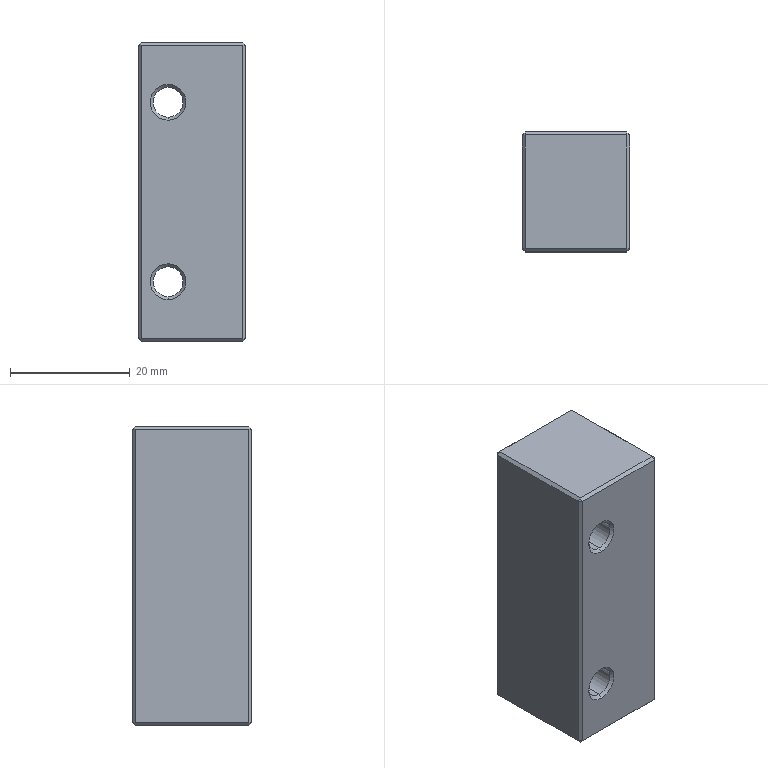Part | SolidWorks | features BaseBody 1 | 1 solid | 38 faces | box 18 x 20 x 50 mm | volume 17163 mm3 | plane 26 | cone 8 | cylinder 4 | commonest cylinder face diameters 5 x4
STEP:
#1=CARTESIAN_POINT('',(-32.,551.5,17.5));
#2=VERTEX_POINT('',#1);
#3=CARTESIAN_POINT('',(-32.,551.5,12.5));
#4=VERTEX_POINT('',#3);
#5=CARTESIAN_POINT('',(-32.,551.5,15.));
#6=DIRECTION('',(0.,-1.,0.));
#7=DIRECTION('',(0.,0.,1.));
#8=AXIS2_PLACEMENT_3D('',#5,#6,#7);
#9=CIRCLE('',#8,2.5);
#10=EDGE_CURVE('',#2,#4,#9,.T.);
#11=ORIENTED_EDGE('',*,*,#10,.F.);
#12=CARTESIAN_POINT('',(-32.,551.,18.));
#13=VERTEX_POINT('',#12);
#14=CARTESIAN_POINT('',(-32.,551.,18.));
#15=DIRECTION('',(0.,-0.7071,0.7071));
#16=VECTOR('',#15,1000.);
#17=LINE('',#14,#16);
#18=EDGE_CURVE('',#2,#13,#17,.T.);
#19=ORIENTED_EDGE('',*,*,#18,.T.);
#20=CARTESIAN_POINT('',(-32.,551.,12.));
#21=VERTEX_POINT('',#20);
#22=CARTESIAN_POINT('',(-32.,551.,15.));
#23=DIRECTION('',(0.,1.,0.));
#24=DIRECTION('',(0.,0.,1.));
#25=AXIS2_PLACEMENT_3D('',#22,#23,#24);
#26=CIRCLE('',#25,3.);
#27=EDGE_CURVE('',#21,#13,#26,.T.);
#28=ORIENTED_EDGE('',*,*,#27,.F.);
#29=CARTESIAN_POINT('',(-32.,551.,12.));
#30=DIRECTION('',(0.,-0.7071,-0.7071));
#31=VECTOR('',#30,1000.);
#32=LINE('',#29,#31);
#33=EDGE_CURVE('',#4,#21,#32,.T.);
#34=ORIENTED_EDGE('',*,*,#33,.F.);
#35=EDGE_LOOP('',(#11,#19,#28,#34));
#36=FACE_OUTER_BOUND('',#35,.T.);
#37=CARTESIAN_POINT('',(-32.,551.,15.));
#38=DIRECTION('',(0.,-1.,0.));
#39=DIRECTION('',(0.,0.,-1.));
#40=AXIS2_PLACEMENT_3D('',#37,#38,#39);
#41=CONICAL_SURFACE('',#40,3.,0.7854);
#42=ADVANCED_FACE('',(#36),#41,.F.);
#43=CARTESIAN_POINT('',(-32.,570.5,12.5));
#44=VERTEX_POINT('',#43);
#45=CARTESIAN_POINT('',(-32.,570.5,17.5));
#46=VERTEX_POINT('',#45);
#47=CARTESIAN_POINT('',(-32.,570.5,15.));
#48=DIRECTION('',(0.,1.,0.));
#49=DIRECTION('',(0.,0.,-1.));
#50=AXIS2_PLACEMENT_3D('',#47,#48,#49);
#51=CIRCLE('',#50,2.5);
#52=EDGE_CURVE('',#44,#46,#51,.T.);
#53=ORIENTED_EDGE('',*,*,#52,.F.);
#54=CARTESIAN_POINT('',(-32.,571.,12.));
#55=VERTEX_POINT('',#54);
#56=CARTESIAN_POINT('',(-32.,570.5,12.5));
#57=DIRECTION('',(0.,0.7071,-0.7071));
#58=VECTOR('',#57,1000.);
#59=LINE('',#56,#58);
#60=EDGE_CURVE('',#44,#55,#59,.T.);
#61=ORIENTED_EDGE('',*,*,#60,.T.);
#62=CARTESIAN_POINT('',(-32.,571.,18.));
#63=VERTEX_POINT('',#62);
#64=CARTESIAN_POINT('',(-32.,571.,15.));
#65=DIRECTION('',(0.,-1.,0.));
#66=DIRECTION('',(0.,0.,-1.));
#67=AXIS2_PLACEMENT_3D('',#64,#65,#66);
#68=CIRCLE('',#67,3.);
#69=EDGE_CURVE('',#63,#55,#68,.T.);
#70=ORIENTED_EDGE('',*,*,#69,.F.);
#71=CARTESIAN_POINT('',(-32.,570.5,17.5));
#72=DIRECTION('',(0.,0.7071,0.7071));
#73=VECTOR('',#72,1000.);
#74=LINE('',#71,#73);
#75=EDGE_CURVE('',#46,#63,#74,.T.);
#76=ORIENTED_EDGE('',*,*,#75,.F.);
#77=EDGE_LOOP('',(#53,#61,#70,#76));
#78=FACE_OUTER_BOUND('',#77,.T.);
#79=CARTESIAN_POINT('',(-32.,570.5,15.));
#80=DIRECTION('',(0.,1.,0.));
#81=DIRECTION('',(0.,0.,1.));
#82=AXIS2_PLACEMENT_3D('',#79,#80,#81);
#83=CONICAL_SURFACE('',#82,2.5,0.7854);
#84=ADVANCED_FACE('',(#78),#83,.F.);
#85=CARTESIAN_POINT('',(-32.,570.5,-17.5));
#86=VERTEX_POINT('',#85);
#87=CARTESIAN_POINT('',(-32.,570.5,-12.5));
#88=VERTEX_POINT('',#87);
#89=CARTESIAN_POINT('',(-32.,570.5,-15.));
#90=DIRECTION('',(0.,1.,0.));
#91=DIRECTION('',(0.,0.,-1.));
#92=AXIS2_PLACEMENT_3D('',#89,#90,#91);
#93=CIRCLE('',#92,2.5);
#94=EDGE_CURVE('',#86,#88,#93,.T.);
#95=ORIENTED_EDGE('',*,*,#94,.F.);
#96=CARTESIAN_POINT('',(-32.,571.,-18.));
#97=VERTEX_POINT('',#96);
#98=CARTESIAN_POINT('',(-32.,570.5,-17.5));
#99=DIRECTION('',(0.,0.7071,-0.7071));
#100=VECTOR('',#99,1000.);
#101=LINE('',#98,#100);
#102=EDGE_CURVE('',#86,#97,#101,.T.);
#103=ORIENTED_EDGE('',*,*,#102,.T.);
#104=CARTESIAN_POINT('',(-32.,571.,-12.));
#105=VERTEX_POINT('',#104);
#106=CARTESIAN_POINT('',(-32.,571.,-15.));
#107=DIRECTION('',(0.,-1.,0.));
#108=DIRECTION('',(0.,0.,-1.));
#109=AXIS2_PLACEMENT_3D('',#106,#107,#108);
#110=CIRCLE('',#109,3.);
#111=EDGE_CURVE('',#105,#97,#110,.T.);
#112=ORIENTED_EDGE('',*,*,#111,.F.);
#113=CARTESIAN_POINT('',(-32.,570.5,-12.5));
#114=DIRECTION('',(0.,0.7071,0.7071));
#115=VECTOR('',#114,1000.);
#116=LINE('',#113,#115);
#117=EDGE_CURVE('',#88,#105,#116,.T.);
#118=ORIENTED_EDGE('',*,*,#117,.F.);
#119=EDGE_LOOP('',(#95,#103,#112,#118));
#120=FACE_OUTER_BOUND('',#119,.T.);
#121=CARTESIAN_POINT('',(-32.,570.5,-15.));
#122=DIRECTION('',(0.,1.,0.));
#123=DIRECTION('',(0.,0.,1.));
#124=AXIS2_PLACEMENT_3D('',#121,#122,#123);
#125=CONICAL_SURFACE('',#124,2.5,0.7854);
#126=ADVANCED_FACE('',(#120),#125,.F.);
#127=CARTESIAN_POINT('',(-32.,551.5,-12.5));
#128=VERTEX_POINT('',#127);
#129=CARTESIAN_POINT('',(-32.,551.5,-17.5));
#130=VERTEX_POINT('',#129);
#131=CARTESIAN_POINT('',(-32.,551.5,-15.));
#132=DIRECTION('',(0.,-1.,0.));
#133=DIRECTION('',(0.,0.,1.));
#134=AXIS2_PLACEMENT_3D('',#131,#132,#133);
#135=CIRCLE('',#134,2.5);
#136=EDGE_CURVE('',#128,#130,#135,.T.);
#137=ORIENTED_EDGE('',*,*,#136,.F.);
#138=CARTESIAN_POINT('',(-32.,551.,-12.));
#139=VERTEX_POINT('',#138);
#140=CARTESIAN_POINT('',(-32.,551.,-12.));
#141=DIRECTION('',(0.,-0.7071,0.7071));
#142=VECTOR('',#141,1000.);
#143=LINE('',#140,#142);
#144=EDGE_CURVE('',#128,#139,#143,.T.);
#145=ORIENTED_EDGE('',*,*,#144,.T.);
#146=CARTESIAN_POINT('',(-32.,551.,-18.));
#147=VERTEX_POINT('',#146);
#148=CARTESIAN_POINT('',(-32.,551.,-15.));
#149=DIRECTION('',(0.,1.,0.));
#150=DIRECTION('',(0.,0.,1.));
#151=AXIS2_PLACEMENT_3D('',#148,#149,#150);
#152=CIRCLE('',#151,3.);
#153=EDGE_CURVE('',#147,#139,#152,.T.);
#154=ORIENTED_EDGE('',*,*,#153,.F.);
#155=CARTESIAN_POINT('',(-32.,551.,-18.));
#156=DIRECTION('',(0.,-0.7071,-0.7071));
#157=VECTOR('',#156,1000.);
#158=LINE('',#155,#157);
#159=EDGE_CURVE('',#130,#147,#158,.T.);
#160=ORIENTED_EDGE('',*,*,#159,.F.);
#161=EDGE_LOOP('',(#137,#145,#154,#160));
#162=FACE_OUTER_BOUND('',#161,.T.);
#163=CARTESIAN_POINT('',(-32.,551.,-15.));
#164=DIRECTION('',(0.,-1.,0.));
#165=DIRECTION('',(0.,0.,-1.));
#166=AXIS2_PLACEMENT_3D('',#163,#164,#165);
#167=CONICAL_SURFACE('',#166,3.,0.7854);
#168=ADVANCED_FACE('',(#162),#167,.F.);
#169=ORIENTED_EDGE('',*,*,#136,.T.);
#170=CARTESIAN_POINT('',(-32.,571.,-17.5));
#171=DIRECTION('',(0.,1.,0.));
#172=VECTOR('',#171,1000.);
#173=LINE('',#170,#172);
#174=EDGE_CURVE('',#130,#86,#173,.T.);
#175=ORIENTED_EDGE('',*,*,#174,.T.);
#176=ORIENTED_EDGE('',*,*,#94,.T.);
#177=CARTESIAN_POINT('',(-32.,571.,-12.5));
#178=DIRECTION('',(0.,1.,0.));
#179=VECTOR('',#178,1000.);
#180=LINE('',#177,#179);
#181=EDGE_CURVE('',#128,#88,#180,.T.);
#182=ORIENTED_EDGE('',*,*,#181,.F.);
#183=EDGE_LOOP('',(#169,#175,#176,#182));
#184=FACE_OUTER_BOUND('',#183,.T.);
#185=CARTESIAN_POINT('',(-32.,571.,-15.));
#186=DIRECTION('',(0.,1.,0.));
#187=DIRECTION('',(0.,0.,1.));
#188=AXIS2_PLACEMENT_3D('',#185,#186,#187);
#189=CYLINDRICAL_SURFACE('',#188,2.5);
#190=ADVANCED_FACE('',(#184),#189,.F.);
#191=ORIENTED_EDGE('',*,*,#10,.T.);
#192=CARTESIAN_POINT('',(-32.,571.,12.5));
#193=DIRECTION('',(0.,1.,0.));
#194=VECTOR('',#193,1000.);
#195=LINE('',#192,#194);
#196=EDGE_CURVE('',#4,#44,#195,.T.);
#197=ORIENTED_EDGE('',*,*,#196,.T.);
#198=ORIENTED_EDGE('',*,*,#52,.T.);
#199=CARTESIAN_POINT('',(-32.,571.,17.5));
#200=DIRECTION('',(0.,1.,0.));
#201=VECTOR('',#200,1000.);
#202=LINE('',#199,#201);
#203=EDGE_CURVE('',#2,#46,#202,.T.);
#204=ORIENTED_EDGE('',*,*,#203,.F.);
#205=EDGE_LOOP('',(#191,#197,#198,#204));
#206=FACE_OUTER_BOUND('',#205,.T.);
#207=CARTESIAN_POINT('',(-32.,571.,15.));
#208=DIRECTION('',(0.,1.,0.));
#209=DIRECTION('',(0.,0.,1.));
#210=AXIS2_PLACEMENT_3D('',#207,#208,#209);
#211=CYLINDRICAL_SURFACE('',#210,2.5);
#212=ADVANCED_FACE('',(#206),#211,.F.);
#213=CARTESIAN_POINT('',(-19.5,551.5,25.));
#214=VERTEX_POINT('',#213);
#215=CARTESIAN_POINT('',(-19.,551.5,24.5));
#216=VERTEX_POINT('',#215);
#217=CARTESIAN_POINT('',(-19.,551.5,24.5));
#218=DIRECTION('',(0.7071,0.,-0.7071));
#219=VECTOR('',#218,1000.);
#220=LINE('',#217,#219);
#221=EDGE_CURVE('',#214,#216,#220,.T.);
#222=ORIENTED_EDGE('',*,*,#221,.T.);
#223=CARTESIAN_POINT('',(-19.,570.5,24.5));
#224=VERTEX_POINT('',#223);
#225=CARTESIAN_POINT('',(-19.,551.,24.5));
#226=DIRECTION('',(0.,-1.,0.));
#227=VECTOR('',#226,1000.);
#228=LINE('',#225,#227);
#229=EDGE_CURVE('',#224,#216,#228,.T.);
#230=ORIENTED_EDGE('',*,*,#229,.F.);
#231=CARTESIAN_POINT('',(-19.5,570.5,25.));
#232=VERTEX_POINT('',#231);
#233=CARTESIAN_POINT('',(-19.5,570.5,25.));
#234=DIRECTION('',(-0.7071,0.,0.7071));
#235=VECTOR('',#234,1000.);
#236=LINE('',#233,#235);
#237=EDGE_CURVE('',#224,#232,#236,.T.);
#238=ORIENTED_EDGE('',*,*,#237,.T.);
#239=CARTESIAN_POINT('',(-19.5,571.,25.));
#240=DIRECTION('',(0.,1.,0.));
#241=VECTOR('',#240,1000.);
#242=LINE('',#239,#241);
#243=EDGE_CURVE('',#214,#232,#242,.T.);
#244=ORIENTED_EDGE('',*,*,#243,.F.);
#245=EDGE_LOOP('',(#222,#230,#238,#244));
#246=FACE_OUTER_BOUND('',#245,.T.);
#247=CARTESIAN_POINT('',(-19.5,571.,25.));
#248=DIRECTION('',(0.7071,0.,0.7071));
#249=DIRECTION('',(0.,-1.,0.));
#250=AXIS2_PLACEMENT_3D('',#247,#248,#249);
#251=PLANE('',#250);
#252=ADVANCED_FACE('',(#246),#251,.T.);
#253=CARTESIAN_POINT('',(-19.5,571.,24.5));
#254=VERTEX_POINT('',#253);
#255=CARTESIAN_POINT('',(-19.25,570.75,24.5));
#256=DIRECTION('',(-0.7071,0.7071,0.));
#257=VECTOR('',#256,1000.);
#258=LINE('',#255,#257);
#259=EDGE_CURVE('',#224,#254,#258,.T.);
#260=ORIENTED_EDGE('',*,*,#259,.T.);
#261=CARTESIAN_POINT('',(-19.5,570.5,25.));
#262=DIRECTION('',(0.,-0.7071,0.7071));
#263=VECTOR('',#262,1000.);
#264=LINE('',#261,#263);
#265=EDGE_CURVE('',#254,#232,#264,.T.);
#266=ORIENTED_EDGE('',*,*,#265,.T.);
#267=ORIENTED_EDGE('',*,*,#237,.F.);
#268=EDGE_LOOP('',(#260,#266,#267));
#269=FACE_OUTER_BOUND('',#268,.T.);
#270=CARTESIAN_POINT('',(-19.5,570.5,25.));
#271=DIRECTION('',(0.5774,0.5774,0.5774));
#272=DIRECTION('',(0.7071,0.,-0.7071));
#273=AXIS2_PLACEMENT_3D('',#270,#271,#272);
#274=PLANE('',#273);
#275=ADVANCED_FACE('',(#269),#274,.T.);
#276=CARTESIAN_POINT('',(-19.5,551.,24.5));
#277=VERTEX_POINT('',#276);
#278=CARTESIAN_POINT('',(-19.5,551.25,24.75));
#279=DIRECTION('',(0.,-0.7071,-0.7071));
#280=VECTOR('',#279,1000.);
#281=LINE('',#278,#280);
#282=EDGE_CURVE('',#214,#277,#281,.T.);
#283=ORIENTED_EDGE('',*,*,#282,.T.);
#284=CARTESIAN_POINT('',(-19.,551.5,24.5));
#285=DIRECTION('',(0.7071,0.7071,0.));
#286=VECTOR('',#285,1000.);
#287=LINE('',#284,#286);
#288=EDGE_CURVE('',#277,#216,#287,.T.);
#289=ORIENTED_EDGE('',*,*,#288,.T.);
#290=ORIENTED_EDGE('',*,*,#221,.F.);
#291=EDGE_LOOP('',(#283,#289,#290));
#292=FACE_OUTER_BOUND('',#291,.T.);
#293=CARTESIAN_POINT('',(-19.,551.5,24.5));
#294=DIRECTION('',(0.5774,-0.5774,0.5774));
#295=DIRECTION('',(0.,-0.7071,-0.7071));
#296=AXIS2_PLACEMENT_3D('',#293,#294,#295);
#297=PLANE('',#296);
#298=ADVANCED_FACE('',(#292),#297,.T.);
#299=CARTESIAN_POINT('',(-19.,570.5,-24.5));
#300=VERTEX_POINT('',#299);
#301=CARTESIAN_POINT('',(-19.5,571.,-24.5));
#302=VERTEX_POINT('',#301);
#303=CARTESIAN_POINT('',(-19.,570.5,-24.5));
#304=DIRECTION('',(-0.7071,0.7071,0.));
#305=VECTOR('',#304,1000.);
#306=LINE('',#303,#305);
#307=EDGE_CURVE('',#300,#302,#306,.T.);
#308=ORIENTED_EDGE('',*,*,#307,.T.);
#309=CARTESIAN_POINT('',(-19.5,571.,-25.));
#310=DIRECTION('',(0.,0.,-1.));
#311=VECTOR('',#310,1000.);
#312=LINE('',#309,#311);
#313=EDGE_CURVE('',#254,#302,#312,.T.);
#314=ORIENTED_EDGE('',*,*,#313,.F.);
#315=ORIENTED_EDGE('',*,*,#259,.F.);
#316=CARTESIAN_POINT('',(-19.,570.5,25.));
#317=DIRECTION('',(0.,0.,1.));
#318=VECTOR('',#317,1000.);
#319=LINE('',#316,#318);
#320=EDGE_CURVE('',#300,#224,#319,.T.);
#321=ORIENTED_EDGE('',*,*,#320,.F.);
#322=EDGE_LOOP('',(#308,#314,#315,#321));
#323=FACE_OUTER_BOUND('',#322,.T.);
#324=CARTESIAN_POINT('',(-19.5,571.,25.));
#325=DIRECTION('',(0.7071,0.7071,0.));
#326=DIRECTION('',(0.,0.,-1.));
#327=AXIS2_PLACEMENT_3D('',#324,#325,#326);
#328=PLANE('',#327);
#329=ADVANCED_FACE('',(#323),#328,.T.);
#330=CARTESIAN_POINT('',(-36.5,571.,24.5));
#331=VERTEX_POINT('',#330);
#332=CARTESIAN_POINT('',(-36.5,570.5,25.));
#333=VERTEX_POINT('',#332);
#334=CARTESIAN_POINT('',(-36.5,571.,24.5));
#335=DIRECTION('',(0.,-0.7071,0.7071));
#336=VECTOR('',#335,1000.);
#337=LINE('',#334,#336);
#338=EDGE_CURVE('',#331,#333,#337,.T.);
#339=ORIENTED_EDGE('',*,*,#338,.T.);
#340=CARTESIAN_POINT('',(-31.,570.5,25.));
#341=DIRECTION('',(-1.,0.,0.));
#342=VECTOR('',#341,1000.);
#343=LINE('',#340,#342);
#344=EDGE_CURVE('',#232,#333,#343,.T.);
#345=ORIENTED_EDGE('',*,*,#344,.F.);
#346=ORIENTED_EDGE('',*,*,#265,.F.);
#347=CARTESIAN_POINT('',(-31.,571.,24.5));
#348=DIRECTION('',(1.,0.,0.));
#349=VECTOR('',#348,1000.);
#350=LINE('',#347,#349);
#351=EDGE_CURVE('',#331,#254,#350,.T.);
#352=ORIENTED_EDGE('',*,*,#351,.F.);
#353=EDGE_LOOP('',(#339,#345,#346,#352));
#354=FACE_OUTER_BOUND('',#353,.T.);
#355=CARTESIAN_POINT('',(-31.,571.,24.5));
#356=DIRECTION('',(0.,-0.7071,-0.7071));
#357=DIRECTION('',(0.,0.7071,-0.7071));
#358=AXIS2_PLACEMENT_3D('',#355,#356,#357);
#359=PLANE('',#358);
#360=ADVANCED_FACE('',(#354),#359,.F.);
#361=CARTESIAN_POINT('',(-36.5,551.5,25.));
#362=VERTEX_POINT('',#361);
#363=CARTESIAN_POINT('',(-36.5,551.,24.5));
#364=VERTEX_POINT('',#363);
#365=CARTESIAN_POINT('',(-36.5,551.25,24.75));
#366=DIRECTION('',(0.,-0.7071,-0.7071));
#367=VECTOR('',#366,1000.);
#368=LINE('',#365,#367);
#369=EDGE_CURVE('',#362,#364,#368,.T.);
#370=ORIENTED_EDGE('',*,*,#369,.T.);
#371=CARTESIAN_POINT('',(-31.,551.,24.5));
#372=DIRECTION('',(-1.,0.,0.));
#373=VECTOR('',#372,1000.);
#374=LINE('',#371,#373);
#375=EDGE_CURVE('',#277,#364,#374,.T.);
#376=ORIENTED_EDGE('',*,*,#375,.F.);
#377=ORIENTED_EDGE('',*,*,#282,.F.);
#378=CARTESIAN_POINT('',(-31.,551.5,25.));
#379=DIRECTION('',(1.,0.,0.));
#380=VECTOR('',#379,1000.);
#381=LINE('',#378,#380);
#382=EDGE_CURVE('',#362,#214,#381,.T.);
#383=ORIENTED_EDGE('',*,*,#382,.F.);
#384=EDGE_LOOP('',(#370,#376,#377,#383));
#385=FACE_OUTER_BOUND('',#384,.T.);
#386=CARTESIAN_POINT('',(-31.,551.5,25.));
#387=DIRECTION('',(0.,0.7071,-0.7071));
#388=DIRECTION('',(-1.,0.,0.));
#389=AXIS2_PLACEMENT_3D('',#386,#387,#388);
#390=PLANE('',#389);
#391=ADVANCED_FACE('',(#385),#390,.F.);
#392=CARTESIAN_POINT('',(-19.5,551.,-24.5));
#393=VERTEX_POINT('',#392);
#394=CARTESIAN_POINT('',(-19.,551.5,-24.5));
#395=VERTEX_POINT('',#394);
#396=CARTESIAN_POINT('',(-19.,551.5,-24.5));
#397=DIRECTION('',(0.7071,0.7071,0.));
#398=VECTOR('',#397,1000.);
#399=LINE('',#396,#398);
#400=EDGE_CURVE('',#393,#395,#399,.T.);
#401=ORIENTED_EDGE('',*,*,#400,.T.);
#402=CARTESIAN_POINT('',(-19.,551.5,-25.));
#403=DIRECTION('',(0.,0.,-1.));
#404=VECTOR('',#403,1000.);
#405=LINE('',#402,#404);
#406=EDGE_CURVE('',#216,#395,#405,.T.);
#407=ORIENTED_EDGE('',*,*,#406,.F.);
#408=ORIENTED_EDGE('',*,*,#288,.F.);
#409=CARTESIAN_POINT('',(-19.5,551.,25.));
#410=DIRECTION('',(0.,0.,1.));
#411=VECTOR('',#410,1000.);
#412=LINE('',#409,#411);
#413=EDGE_CURVE('',#393,#277,#412,.T.);
#414=ORIENTED_EDGE('',*,*,#413,.F.);
#415=EDGE_LOOP('',(#401,#407,#408,#414));
#416=FACE_OUTER_BOUND('',#415,.T.);
#417=CARTESIAN_POINT('',(-19.5,551.,25.));
#418=DIRECTION('',(0.7071,-0.7071,0.));
#419=DIRECTION('',(0.,0.,-1.));
#420=AXIS2_PLACEMENT_3D('',#417,#418,#419);
#421=PLANE('',#420);
#422=ADVANCED_FACE('',(#416),#421,.T.);
#423=CARTESIAN_POINT('',(-19.5,570.5,-25.));
#424=VERTEX_POINT('',#423);
#425=CARTESIAN_POINT('',(-19.,570.5,-24.5));
#426=DIRECTION('',(-0.7071,0.,-0.7071));
#427=VECTOR('',#426,1000.);
#428=LINE('',#425,#427);
#429=EDGE_CURVE('',#300,#424,#428,.T.);
#430=ORIENTED_EDGE('',*,*,#429,.T.);
#431=CARTESIAN_POINT('',(-19.5,570.75,-24.75));
#432=DIRECTION('',(0.,0.7071,0.7071));
#433=VECTOR('',#432,1000.);
#434=LINE('',#431,#433);
#435=EDGE_CURVE('',#424,#302,#434,.T.);
#436=ORIENTED_EDGE('',*,*,#435,.T.);
#437=ORIENTED_EDGE('',*,*,#307,.F.);
#438=EDGE_LOOP('',(#430,#436,#437));
#439=FACE_OUTER_BOUND('',#438,.T.);
#440=CARTESIAN_POINT('',(-19.,570.5,-24.5));
#441=DIRECTION('',(0.5774,0.5774,-0.5774));
#442=DIRECTION('',(-0.7071,0.,-0.7071));
#443=AXIS2_PLACEMENT_3D('',#440,#441,#442);
#444=PLANE('',#443);
#445=ADVANCED_FACE('',(#439),#444,.T.);
#446=CARTESIAN_POINT('',(-37.,570.5,24.5));
#447=VERTEX_POINT('',#446);
#448=CARTESIAN_POINT('',(-36.5,571.,24.5));
#449=DIRECTION('',(-0.7071,-0.7071,0.));
#450=VECTOR('',#449,1000.);
#451=LINE('',#448,#450);
#452=EDGE_CURVE('',#331,#447,#451,.T.);
#453=ORIENTED_EDGE('',*,*,#452,.T.);
#454=CARTESIAN_POINT('',(-36.75,570.5,24.75));
#455=DIRECTION('',(0.7071,0.,0.7071));
#456=VECTOR('',#455,1000.);
#457=LINE('',#454,#456);
#458=EDGE_CURVE('',#447,#333,#457,.T.);
#459=ORIENTED_EDGE('',*,*,#458,.T.);
#460=ORIENTED_EDGE('',*,*,#338,.F.);
#461=EDGE_LOOP('',(#453,#459,#460));
#462=FACE_OUTER_BOUND('',#461,.T.);
#463=CARTESIAN_POINT('',(-36.5,571.,24.5));
#464=DIRECTION('',(-0.5774,0.5774,0.5774));
#465=DIRECTION('',(0.7071,0.,0.7071));
#466=AXIS2_PLACEMENT_3D('',#463,#464,#465);
#467=PLANE('',#466);
#468=ADVANCED_FACE('',(#462),#467,.T.);
#469=CARTESIAN_POINT('',(-37.,551.5,24.5));
#470=VERTEX_POINT('',#469);
#471=CARTESIAN_POINT('',(-37.,551.5,24.5));
#472=DIRECTION('',(-0.7071,0.,-0.7071));
#473=VECTOR('',#472,1000.);
#474=LINE('',#471,#473);
#475=EDGE_CURVE('',#362,#470,#474,.T.);
#476=ORIENTED_EDGE('',*,*,#475,.T.);
#477=CARTESIAN_POINT('',(-37.,551.5,24.5));
#478=DIRECTION('',(0.7071,-0.7071,0.));
#479=VECTOR('',#478,1000.);
#480=LINE('',#477,#479);
#481=EDGE_CURVE('',#470,#364,#480,.T.);
#482=ORIENTED_EDGE('',*,*,#481,.T.);
#483=ORIENTED_EDGE('',*,*,#369,.F.);
#484=EDGE_LOOP('',(#476,#482,#483));
#485=FACE_OUTER_BOUND('',#484,.T.);
#486=CARTESIAN_POINT('',(-37.,551.5,24.5));
#487=DIRECTION('',(-0.5774,-0.5774,0.5774));
#488=DIRECTION('',(-0.7071,0.7071,0.));
#489=AXIS2_PLACEMENT_3D('',#486,#487,#488);
#490=PLANE('',#489);
#491=ADVANCED_FACE('',(#485),#490,.T.);
#492=CARTESIAN_POINT('',(-19.5,551.5,-25.));
#493=VERTEX_POINT('',#492);
#494=CARTESIAN_POINT('',(-19.5,551.25,-24.75));
#495=DIRECTION('',(0.,0.7071,-0.7071));
#496=VECTOR('',#495,1000.);
#497=LINE('',#494,#496);
#498=EDGE_CURVE('',#393,#493,#497,.T.);
#499=ORIENTED_EDGE('',*,*,#498,.T.);
#500=CARTESIAN_POINT('',(-19.,551.5,-24.5));
#501=DIRECTION('',(0.7071,0.,0.7071));
#502=VECTOR('',#501,1000.);
#503=LINE('',#500,#502);
#504=EDGE_CURVE('',#493,#395,#503,.T.);
#505=ORIENTED_EDGE('',*,*,#504,.T.);
#506=ORIENTED_EDGE('',*,*,#400,.F.);
#507=EDGE_LOOP('',(#499,#505,#506));
#508=FACE_OUTER_BOUND('',#507,.T.);
#509=CARTESIAN_POINT('',(-19.,551.5,-24.5));
#510=DIRECTION('',(0.5774,-0.5774,-0.5774));
#511=DIRECTION('',(0.,0.7071,-0.7071));
#512=AXIS2_PLACEMENT_3D('',#509,#510,#511);
#513=PLANE('',#512);
#514=ADVANCED_FACE('',(#508),#513,.T.);
#515=ORIENTED_EDGE('',*,*,#504,.F.);
#516=CARTESIAN_POINT('',(-19.5,551.,-25.));
#517=DIRECTION('',(0.,-1.,0.));
#518=VECTOR('',#517,1000.);
#519=LINE('',#516,#518);
#520=EDGE_CURVE('',#424,#493,#519,.T.);
#521=ORIENTED_EDGE('',*,*,#520,.F.);
#522=ORIENTED_EDGE('',*,*,#429,.F.);
#523=CARTESIAN_POINT('',(-19.,571.,-24.5));
#524=DIRECTION('',(0.,1.,0.));
#525=VECTOR('',#524,1000.);
#526=LINE('',#523,#525);
#527=EDGE_CURVE('',#395,#300,#526,.T.);
#528=ORIENTED_EDGE('',*,*,#527,.F.);
#529=EDGE_LOOP('',(#515,#521,#522,#528));
#530=FACE_OUTER_BOUND('',#529,.T.);
#531=CARTESIAN_POINT('',(-19.5,571.,-25.));
#532=DIRECTION('',(0.7071,0.,-0.7071));
#533=DIRECTION('',(0.,-1.,0.));
#534=AXIS2_PLACEMENT_3D('',#531,#532,#533);
#535=PLANE('',#534);
#536=ADVANCED_FACE('',(#530),#535,.T.);
#537=CARTESIAN_POINT('',(-36.5,570.5,-25.));
#538=VERTEX_POINT('',#537);
#539=CARTESIAN_POINT('',(-36.5,571.,-24.5));
#540=VERTEX_POINT('',#539);
#541=CARTESIAN_POINT('',(-36.5,570.5,-25.));
#542=DIRECTION('',(0.,0.7071,0.7071));
#543=VECTOR('',#542,1000.);
#544=LINE('',#541,#543);
#545=EDGE_CURVE('',#538,#540,#544,.T.);
#546=ORIENTED_EDGE('',*,*,#545,.T.);
#547=CARTESIAN_POINT('',(-31.,571.,-24.5));
#548=DIRECTION('',(-1.,0.,0.));
#549=VECTOR('',#548,1000.);
#550=LINE('',#547,#549);
#551=EDGE_CURVE('',#302,#540,#550,.T.);
#552=ORIENTED_EDGE('',*,*,#551,.F.);
#553=ORIENTED_EDGE('',*,*,#435,.F.);
#554=CARTESIAN_POINT('',(-31.,570.5,-25.));
#555=DIRECTION('',(1.,0.,0.));
#556=VECTOR('',#555,1000.);
#557=LINE('',#554,#556);
#558=EDGE_CURVE('',#538,#424,#557,.T.);
#559=ORIENTED_EDGE('',*,*,#558,.F.);
#560=EDGE_LOOP('',(#546,#552,#553,#559));
#561=FACE_OUTER_BOUND('',#560,.T.);
#562=CARTESIAN_POINT('',(-31.,570.5,-25.));
#563=DIRECTION('',(0.,-0.7071,0.7071));
#564=DIRECTION('',(-1.,0.,0.));
#565=AXIS2_PLACEMENT_3D('',#562,#563,#564);
#566=PLANE('',#565);
#567=ADVANCED_FACE('',(#561),#566,.F.);
#568=CARTESIAN_POINT('',(-37.,570.5,-24.5));
#569=VERTEX_POINT('',#568);
#570=CARTESIAN_POINT('',(-36.75,570.75,-24.5));
#571=DIRECTION('',(-0.7071,-0.7071,0.));
#572=VECTOR('',#571,1000.);
#573=LINE('',#570,#572);
#574=EDGE_CURVE('',#540,#569,#573,.T.);
#575=ORIENTED_EDGE('',*,*,#574,.T.);
#576=CARTESIAN_POINT('',(-37.,570.5,-25.));
#577=DIRECTION('',(0.,0.,-1.));
#578=VECTOR('',#577,1000.);
#579=LINE('',#576,#578);
#580=EDGE_CURVE('',#447,#569,#579,.T.);
#581=ORIENTED_EDGE('',*,*,#580,.F.);
#582=ORIENTED_EDGE('',*,*,#452,.F.);
#583=CARTESIAN_POINT('',(-36.5,571.,25.));
#584=DIRECTION('',(0.,0.,1.));
#585=VECTOR('',#584,1000.);
#586=LINE('',#583,#585);
#587=EDGE_CURVE('',#540,#331,#586,.T.);
#588=ORIENTED_EDGE('',*,*,#587,.F.);
#589=EDGE_LOOP('',(#575,#581,#582,#588));
#590=FACE_OUTER_BOUND('',#589,.T.);
#591=CARTESIAN_POINT('',(-37.,570.5,0.));
#592=DIRECTION('',(-0.7071,0.7071,0.));
#593=DIRECTION('',(0.,0.,1.));
#594=AXIS2_PLACEMENT_3D('',#591,#592,#593);
#595=PLANE('',#594);
#596=ADVANCED_FACE('',(#590),#595,.T.);
#597=ORIENTED_EDGE('',*,*,#458,.F.);
#598=CARTESIAN_POINT('',(-37.,571.,24.5));
#599=DIRECTION('',(0.,1.,0.));
#600=VECTOR('',#599,1000.);
#601=LINE('',#598,#600);
#602=EDGE_CURVE('',#470,#447,#601,.T.);
#603=ORIENTED_EDGE('',*,*,#602,.F.);
#604=ORIENTED_EDGE('',*,*,#475,.F.);
#605=CARTESIAN_POINT('',(-36.5,551.,25.));
#606=DIRECTION('',(0.,-1.,0.));
#607=VECTOR('',#606,1000.);
#608=LINE('',#605,#607);
#609=EDGE_CURVE('',#333,#362,#608,.T.);
#610=ORIENTED_EDGE('',*,*,#609,.F.);
#611=EDGE_LOOP('',(#597,#603,#604,#610));
#612=FACE_OUTER_BOUND('',#611,.T.);
#613=CARTESIAN_POINT('',(-37.,725.,24.5));
#614=DIRECTION('',(-0.7071,0.,0.7071));
#615=DIRECTION('',(0.,1.,0.));
#616=AXIS2_PLACEMENT_3D('',#613,#614,#615);
#617=PLANE('',#616);
#618=ADVANCED_FACE('',(#612),#617,.T.);
#619=CARTESIAN_POINT('',(-37.,551.5,-24.5));
#620=VERTEX_POINT('',#619);
#621=CARTESIAN_POINT('',(-36.5,551.,-24.5));
#622=VERTEX_POINT('',#621);
#623=CARTESIAN_POINT('',(-36.5,551.,-24.5));
#624=DIRECTION('',(0.7071,-0.7071,0.));
#625=VECTOR('',#624,1000.);
#626=LINE('',#623,#625);
#627=EDGE_CURVE('',#620,#622,#626,.T.);
#628=ORIENTED_EDGE('',*,*,#627,.T.);
#629=CARTESIAN_POINT('',(-36.5,551.,-25.));
#630=DIRECTION('',(0.,0.,-1.));
#631=VECTOR('',#630,1000.);
#632=LINE('',#629,#631);
#633=EDGE_CURVE('',#364,#622,#632,.T.);
#634=ORIENTED_EDGE('',*,*,#633,.F.);
#635=ORIENTED_EDGE('',*,*,#481,.F.);
#636=CARTESIAN_POINT('',(-37.,551.5,25.));
#637=DIRECTION('',(0.,0.,1.));
#638=VECTOR('',#637,1000.);
#639=LINE('',#636,#638);
#640=EDGE_CURVE('',#620,#470,#639,.T.);
#641=ORIENTED_EDGE('',*,*,#640,.F.);
#642=EDGE_LOOP('',(#628,#634,#635,#641));
#643=FACE_OUTER_BOUND('',#642,.T.);
#644=CARTESIAN_POINT('',(-37.,551.5,0.));
#645=DIRECTION('',(-0.7071,-0.7071,0.));
#646=DIRECTION('',(-0.7071,0.7071,0.));
#647=AXIS2_PLACEMENT_3D('',#644,#645,#646);
#648=PLANE('',#647);
#649=ADVANCED_FACE('',(#643),#648,.T.);
#650=CARTESIAN_POINT('',(-36.5,551.5,-25.));
#651=VERTEX_POINT('',#650);
#652=CARTESIAN_POINT('',(-36.5,551.,-24.5));
#653=DIRECTION('',(0.,0.7071,-0.7071));
#654=VECTOR('',#653,1000.);
#655=LINE('',#652,#654);
#656=EDGE_CURVE('',#622,#651,#655,.T.);
#657=ORIENTED_EDGE('',*,*,#656,.T.);
#658=CARTESIAN_POINT('',(-31.,551.5,-25.));
#659=DIRECTION('',(-1.,0.,0.));
#660=VECTOR('',#659,1000.);
#661=LINE('',#658,#660);
#662=EDGE_CURVE('',#493,#651,#661,.T.);
#663=ORIENTED_EDGE('',*,*,#662,.F.);
#664=ORIENTED_EDGE('',*,*,#498,.F.);
#665=CARTESIAN_POINT('',(-31.,551.,-24.5));
#666=DIRECTION('',(1.,0.,0.));
#667=VECTOR('',#666,1000.);
#668=LINE('',#665,#667);
#669=EDGE_CURVE('',#622,#393,#668,.T.);
#670=ORIENTED_EDGE('',*,*,#669,.F.);
#671=EDGE_LOOP('',(#657,#663,#664,#670));
#672=FACE_OUTER_BOUND('',#671,.T.);
#673=CARTESIAN_POINT('',(-31.,551.,-24.5));
#674=DIRECTION('',(0.,0.7071,0.7071));
#675=DIRECTION('',(1.,0.,0.));
#676=AXIS2_PLACEMENT_3D('',#673,#674,#675);
#677=PLANE('',#676);
#678=ADVANCED_FACE('',(#672),#677,.F.);
#679=ORIENTED_EDGE('',*,*,#545,.F.);
#680=CARTESIAN_POINT('',(-36.5,570.5,-25.));
#681=DIRECTION('',(-0.7071,0.,0.7071));
#682=VECTOR('',#681,1000.);
#683=LINE('',#680,#682);
#684=EDGE_CURVE('',#538,#569,#683,.T.);
#685=ORIENTED_EDGE('',*,*,#684,.T.);
#686=ORIENTED_EDGE('',*,*,#574,.F.);
#687=EDGE_LOOP('',(#679,#685,#686));
#688=FACE_OUTER_BOUND('',#687,.T.);
#689=CARTESIAN_POINT('',(-36.5,570.5,-25.));
#690=DIRECTION('',(-0.5774,0.5774,-0.5774));
#691=DIRECTION('',(-0.7071,0.,0.7071));
#692=AXIS2_PLACEMENT_3D('',#689,#690,#691);
#693=PLANE('',#692);
#694=ADVANCED_FACE('',(#688),#693,.T.);
#695=ORIENTED_EDGE('',*,*,#627,.F.);
#696=CARTESIAN_POINT('',(-36.75,551.5,-24.75));
#697=DIRECTION('',(0.7071,0.,-0.7071));
#698=VECTOR('',#697,1000.);
#699=LINE('',#696,#698);
#700=EDGE_CURVE('',#620,#651,#699,.T.);
#701=ORIENTED_EDGE('',*,*,#700,.T.);
#702=ORIENTED_EDGE('',*,*,#656,.F.);
#703=EDGE_LOOP('',(#695,#701,#702));
#704=FACE_OUTER_BOUND('',#703,.T.);
#705=CARTESIAN_POINT('',(-36.5,551.,-24.5));
#706=DIRECTION('',(-0.5774,-0.5774,-0.5774));
#707=DIRECTION('',(-0.7071,0.7071,0.));
#708=AXIS2_PLACEMENT_3D('',#705,#706,#707);
#709=PLANE('',#708);
#710=ADVANCED_FACE('',(#704),#709,.T.);
#711=ORIENTED_EDGE('',*,*,#700,.F.);
#712=CARTESIAN_POINT('',(-37.,551.,-24.5));
#713=DIRECTION('',(0.,-1.,0.));
#714=VECTOR('',#713,1000.);
#715=LINE('',#712,#714);
#716=EDGE_CURVE('',#569,#620,#715,.T.);
#717=ORIENTED_EDGE('',*,*,#716,.F.);
#718=ORIENTED_EDGE('',*,*,#684,.F.);
#719=CARTESIAN_POINT('',(-36.5,571.,-25.));
#720=DIRECTION('',(0.,1.,0.));
#721=VECTOR('',#720,1000.);
#722=LINE('',#719,#721);
#723=EDGE_CURVE('',#651,#538,#722,.T.);
#724=ORIENTED_EDGE('',*,*,#723,.F.);
#725=EDGE_LOOP('',(#711,#717,#718,#724));
#726=FACE_OUTER_BOUND('',#725,.T.);
#727=CARTESIAN_POINT('',(-37.,725.,-24.5));
#728=DIRECTION('',(-0.7071,0.,-0.7071));
#729=DIRECTION('',(-0.7071,0.,0.7071));
#730=AXIS2_PLACEMENT_3D('',#727,#728,#729);
#731=PLANE('',#730);
#732=ADVANCED_FACE('',(#726),#731,.T.);
#733=ORIENTED_EDGE('',*,*,#320,.T.);
#734=ORIENTED_EDGE('',*,*,#229,.T.);
#735=ORIENTED_EDGE('',*,*,#406,.T.);
#736=ORIENTED_EDGE('',*,*,#527,.T.);
#737=EDGE_LOOP('',(#733,#734,#735,#736));
#738=FACE_OUTER_BOUND('',#737,.T.);
#739=CARTESIAN_POINT('',(-19.,0.,0.));
#740=DIRECTION('',(1.,0.,0.));
#741=DIRECTION('',(0.,1.,0.));
#742=AXIS2_PLACEMENT_3D('',#739,#740,#741);
#743=PLANE('',#742);
#744=ADVANCED_FACE('',(#738),#743,.T.);
#745=ORIENTED_EDGE('',*,*,#716,.T.);
#746=ORIENTED_EDGE('',*,*,#640,.T.);
#747=ORIENTED_EDGE('',*,*,#602,.T.);
#748=ORIENTED_EDGE('',*,*,#580,.T.);
#749=EDGE_LOOP('',(#745,#746,#747,#748));
#750=FACE_OUTER_BOUND('',#749,.T.);
#751=CARTESIAN_POINT('',(-37.,725.,0.));
#752=DIRECTION('',(-1.,0.,0.));
#753=DIRECTION('',(0.,0.,1.));
#754=AXIS2_PLACEMENT_3D('',#751,#752,#753);
#755=PLANE('',#754);
#756=ADVANCED_FACE('',(#750),#755,.T.);
#757=ORIENTED_EDGE('',*,*,#27,.T.);
#758=CARTESIAN_POINT('',(-32.,551.,15.));
#759=DIRECTION('',(0.,1.,0.));
#760=DIRECTION('',(0.,0.,1.));
#761=AXIS2_PLACEMENT_3D('',#758,#759,#760);
#762=CIRCLE('',#761,3.);
#763=EDGE_CURVE('',#13,#21,#762,.T.);
#764=ORIENTED_EDGE('',*,*,#763,.T.);
#765=EDGE_LOOP('',(#757,#764));
#766=FACE_BOUND('',#765,.T.);
#767=ORIENTED_EDGE('',*,*,#153,.T.);
#768=CARTESIAN_POINT('',(-32.,551.,-15.));
#769=DIRECTION('',(0.,1.,0.));
#770=DIRECTION('',(0.,0.,1.));
#771=AXIS2_PLACEMENT_3D('',#768,#769,#770);
#772=CIRCLE('',#771,3.);
#773=EDGE_CURVE('',#139,#147,#772,.T.);
#774=ORIENTED_EDGE('',*,*,#773,.T.);
#775=EDGE_LOOP('',(#767,#774));
#776=FACE_BOUND('',#775,.T.);
#777=ORIENTED_EDGE('',*,*,#633,.T.);
#778=ORIENTED_EDGE('',*,*,#669,.T.);
#779=ORIENTED_EDGE('',*,*,#413,.T.);
#780=ORIENTED_EDGE('',*,*,#375,.T.);
#781=EDGE_LOOP('',(#777,#778,#779,#780));
#782=FACE_OUTER_BOUND('',#781,.T.);
#783=CARTESIAN_POINT('',(-31.,551.,25.));
#784=DIRECTION('',(0.,1.,0.));
#785=DIRECTION('',(1.,0.,0.));
#786=AXIS2_PLACEMENT_3D('',#783,#784,#785);
#787=PLANE('',#786);
#788=ADVANCED_FACE('',(#766,#776,#782),#787,.F.);
#789=ORIENTED_EDGE('',*,*,#558,.T.);
#790=ORIENTED_EDGE('',*,*,#520,.T.);
#791=ORIENTED_EDGE('',*,*,#662,.T.);
#792=ORIENTED_EDGE('',*,*,#723,.T.);
#793=EDGE_LOOP('',(#789,#790,#791,#792));
#794=FACE_OUTER_BOUND('',#793,.T.);
#795=CARTESIAN_POINT('',(-31.,571.,-25.));
#796=DIRECTION('',(0.,0.,1.));
#797=DIRECTION('',(1.,0.,0.));
#798=AXIS2_PLACEMENT_3D('',#795,#796,#797);
#799=PLANE('',#798);
#800=ADVANCED_FACE('',(#794),#799,.F.);
#801=ORIENTED_EDGE('',*,*,#69,.T.);
#802=CARTESIAN_POINT('',(-32.,571.,15.));
#803=DIRECTION('',(0.,-1.,0.));
#804=DIRECTION('',(0.,0.,-1.));
#805=AXIS2_PLACEMENT_3D('',#802,#803,#804);
#806=CIRCLE('',#805,3.);
#807=EDGE_CURVE('',#55,#63,#806,.T.);
#808=ORIENTED_EDGE('',*,*,#807,.T.);
#809=EDGE_LOOP('',(#801,#808));
#810=FACE_BOUND('',#809,.T.);
#811=ORIENTED_EDGE('',*,*,#111,.T.);
#812=CARTESIAN_POINT('',(-32.,571.,-15.));
#813=DIRECTION('',(0.,-1.,0.));
#814=DIRECTION('',(0.,0.,-1.));
#815=AXIS2_PLACEMENT_3D('',#812,#813,#814);
#816=CIRCLE('',#815,3.);
#817=EDGE_CURVE('',#97,#105,#816,.T.);
#818=ORIENTED_EDGE('',*,*,#817,.T.);
#819=EDGE_LOOP('',(#811,#818));
#820=FACE_BOUND('',#819,.T.);
#821=ORIENTED_EDGE('',*,*,#351,.T.);
#822=ORIENTED_EDGE('',*,*,#313,.T.);
#823=ORIENTED_EDGE('',*,*,#551,.T.);
#824=ORIENTED_EDGE('',*,*,#587,.T.);
#825=EDGE_LOOP('',(#821,#822,#823,#824));
#826=FACE_OUTER_BOUND('',#825,.T.);
#827=CARTESIAN_POINT('',(-31.,571.,25.));
#828=DIRECTION('',(0.,-1.,0.));
#829=DIRECTION('',(0.,0.,-1.));
#830=AXIS2_PLACEMENT_3D('',#827,#828,#829);
#831=PLANE('',#830);
#832=ADVANCED_FACE('',(#810,#820,#826),#831,.F.);
#833=ORIENTED_EDGE('',*,*,#382,.T.);
#834=ORIENTED_EDGE('',*,*,#243,.T.);
#835=ORIENTED_EDGE('',*,*,#344,.T.);
#836=ORIENTED_EDGE('',*,*,#609,.T.);
#837=EDGE_LOOP('',(#833,#834,#835,#836));
#838=FACE_OUTER_BOUND('',#837,.T.);
#839=CARTESIAN_POINT('',(-31.,571.,25.));
#840=DIRECTION('',(0.,0.,-1.));
#841=DIRECTION('',(0.,-1.,0.));
#842=AXIS2_PLACEMENT_3D('',#839,#840,#841);
#843=PLANE('',#842);
#844=ADVANCED_FACE('',(#838),#843,.F.);
#845=ORIENTED_EDGE('',*,*,#196,.F.);
#846=CARTESIAN_POINT('',(-32.,551.5,15.));
#847=DIRECTION('',(0.,-1.,0.));
#848=DIRECTION('',(0.,0.,1.));
#849=AXIS2_PLACEMENT_3D('',#846,#847,#848);
#850=CIRCLE('',#849,2.5);
#851=EDGE_CURVE('',#4,#2,#850,.T.);
#852=ORIENTED_EDGE('',*,*,#851,.T.);
#853=ORIENTED_EDGE('',*,*,#203,.T.);
#854=CARTESIAN_POINT('',(-32.,570.5,15.));
#855=DIRECTION('',(0.,1.,0.));
#856=DIRECTION('',(0.,0.,-1.));
#857=AXIS2_PLACEMENT_3D('',#854,#855,#856);
#858=CIRCLE('',#857,2.5);
#859=EDGE_CURVE('',#46,#44,#858,.T.);
#860=ORIENTED_EDGE('',*,*,#859,.T.);
#861=EDGE_LOOP('',(#845,#852,#853,#860));
#862=FACE_OUTER_BOUND('',#861,.T.);
#863=CARTESIAN_POINT('',(-32.,571.,15.));
#864=DIRECTION('',(0.,1.,0.));
#865=DIRECTION('',(0.,0.,1.));
#866=AXIS2_PLACEMENT_3D('',#863,#864,#865);
#867=CYLINDRICAL_SURFACE('',#866,2.5);
#868=ADVANCED_FACE('',(#862),#867,.F.);
#869=ORIENTED_EDGE('',*,*,#174,.F.);
#870=CARTESIAN_POINT('',(-32.,551.5,-15.));
#871=DIRECTION('',(0.,-1.,0.));
#872=DIRECTION('',(0.,0.,1.));
#873=AXIS2_PLACEMENT_3D('',#870,#871,#872);
#874=CIRCLE('',#873,2.5);
#875=EDGE_CURVE('',#130,#128,#874,.T.);
#876=ORIENTED_EDGE('',*,*,#875,.T.);
#877=ORIENTED_EDGE('',*,*,#181,.T.);
#878=CARTESIAN_POINT('',(-32.,570.5,-15.));
#879=DIRECTION('',(0.,1.,0.));
#880=DIRECTION('',(0.,0.,-1.));
#881=AXIS2_PLACEMENT_3D('',#878,#879,#880);
#882=CIRCLE('',#881,2.5);
#883=EDGE_CURVE('',#88,#86,#882,.T.);
#884=ORIENTED_EDGE('',*,*,#883,.T.);
#885=EDGE_LOOP('',(#869,#876,#877,#884));
#886=FACE_OUTER_BOUND('',#885,.T.);
#887=CARTESIAN_POINT('',(-32.,571.,-15.));
#888=DIRECTION('',(0.,1.,0.));
#889=DIRECTION('',(0.,0.,1.));
#890=AXIS2_PLACEMENT_3D('',#887,#888,#889);
#891=CYLINDRICAL_SURFACE('',#890,2.5);
#892=ADVANCED_FACE('',(#886),#891,.F.);
#893=ORIENTED_EDGE('',*,*,#144,.F.);
#894=ORIENTED_EDGE('',*,*,#875,.F.);
#895=ORIENTED_EDGE('',*,*,#159,.T.);
#896=ORIENTED_EDGE('',*,*,#773,.F.);
#897=EDGE_LOOP('',(#893,#894,#895,#896));
#898=FACE_OUTER_BOUND('',#897,.T.);
#899=CARTESIAN_POINT('',(-32.,551.,-15.));
#900=DIRECTION('',(0.,-1.,0.));
#901=DIRECTION('',(0.,0.,-1.));
#902=AXIS2_PLACEMENT_3D('',#899,#900,#901);
#903=CONICAL_SURFACE('',#902,3.,0.7854);
#904=ADVANCED_FACE('',(#898),#903,.F.);
#905=ORIENTED_EDGE('',*,*,#102,.F.);
#906=ORIENTED_EDGE('',*,*,#883,.F.);
#907=ORIENTED_EDGE('',*,*,#117,.T.);
#908=ORIENTED_EDGE('',*,*,#817,.F.);
#909=EDGE_LOOP('',(#905,#906,#907,#908));
#910=FACE_OUTER_BOUND('',#909,.T.);
#911=CARTESIAN_POINT('',(-32.,570.5,-15.));
#912=DIRECTION('',(0.,1.,0.));
#913=DIRECTION('',(0.,0.,1.));
#914=AXIS2_PLACEMENT_3D('',#911,#912,#913);
#915=CONICAL_SURFACE('',#914,2.5,0.7854);
#916=ADVANCED_FACE('',(#910),#915,.F.);
#917=ORIENTED_EDGE('',*,*,#60,.F.);
#918=ORIENTED_EDGE('',*,*,#859,.F.);
#919=ORIENTED_EDGE('',*,*,#75,.T.);
#920=ORIENTED_EDGE('',*,*,#807,.F.);
#921=EDGE_LOOP('',(#917,#918,#919,#920));
#922=FACE_OUTER_BOUND('',#921,.T.);
#923=CARTESIAN_POINT('',(-32.,570.5,15.));
#924=DIRECTION('',(0.,1.,0.));
#925=DIRECTION('',(0.,0.,1.));
#926=AXIS2_PLACEMENT_3D('',#923,#924,#925);
#927=CONICAL_SURFACE('',#926,2.5,0.7854);
#928=ADVANCED_FACE('',(#922),#927,.F.);
#929=ORIENTED_EDGE('',*,*,#18,.F.);
#930=ORIENTED_EDGE('',*,*,#851,.F.);
#931=ORIENTED_EDGE('',*,*,#33,.T.);
#932=ORIENTED_EDGE('',*,*,#763,.F.);
#933=EDGE_LOOP('',(#929,#930,#931,#932));
#934=FACE_OUTER_BOUND('',#933,.T.);
#935=CARTESIAN_POINT('',(-32.,551.,15.));
#936=DIRECTION('',(0.,-1.,0.));
#937=DIRECTION('',(0.,0.,-1.));
#938=AXIS2_PLACEMENT_3D('',#935,#936,#937);
#939=CONICAL_SURFACE('',#938,3.,0.7854);
#940=ADVANCED_FACE('',(#934),#939,.F.);
#941=CLOSED_SHELL('',(#42,#84,#126,#168,#190,#212,#252,#275,#298,#329,#360,#391,#422,#445,#468,#491,#514,#536,#567,#596,#618,#649,#678,#694,#710,#732,#744,#756,#788,#800,#832,#844,#868,#892,#904,#916,#928,#940));
#942=MANIFOLD_SOLID_BREP('',#941);
#943=CARTESIAN_POINT('',(0.,0.,0.));
#944=DIRECTION('',(0.,0.,1.));
#945=DIRECTION('',(1.,0.,0.));
#946=AXIS2_PLACEMENT_3D('',#943,#944,#945);
#947=(LENGTH_UNIT()NAMED_UNIT(*)SI_UNIT(.MILLI.,.METRE.));
#948=UNCERTAINTY_MEASURE_WITH_UNIT(LENGTH_MEASURE(0.00001),#947,'','');
#949=(NAMED_UNIT(*)PLANE_ANGLE_UNIT()SI_UNIT($,.RADIAN.));
#950=(NAMED_UNIT(*)SI_UNIT($,.STERADIAN.)SOLID_ANGLE_UNIT());
#951=(GEOMETRIC_REPRESENTATION_CONTEXT(3)GLOBAL_UNCERTAINTY_ASSIGNED_CONTEXT((#948))GLOBAL_UNIT_ASSIGNED_CONTEXT((#947,#949,#950))REPRESENTATION_CONTEXT('',''));
#952=ADVANCED_BREP_SHAPE_REPRESENTATION('',(#942,#946),#951);